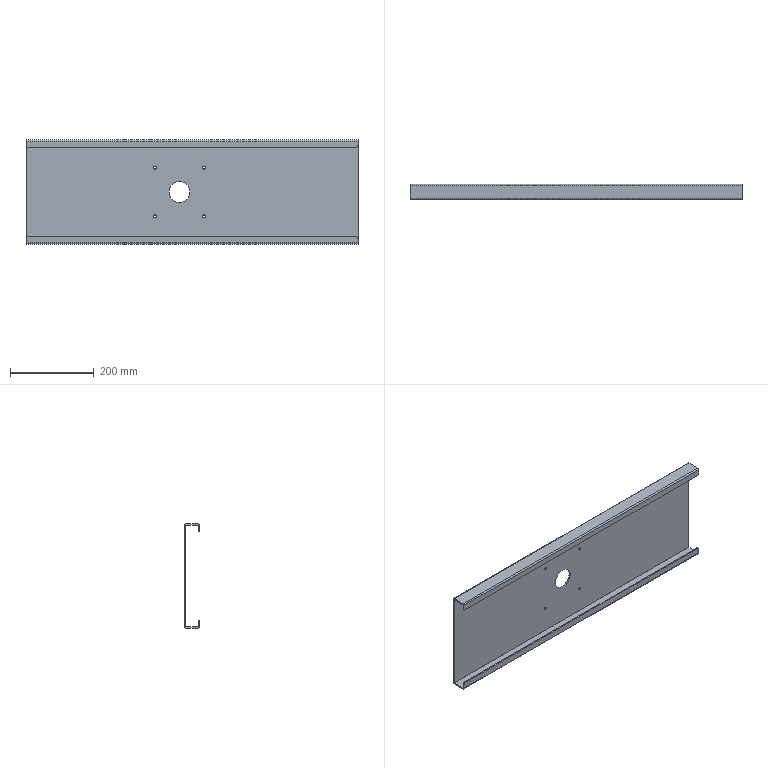Part | STEP file | HESS-408-70-15W-W-38-motor fixing bracket | 1 solid | 36 faces | box 795 x 36 x 250 mm | volume 812268 mm3 | cylinder 22 | plane 14 | commonest cylinder face diameters 6.8 x8 0.2 x4 6.2 x4 10 x4 50 x2